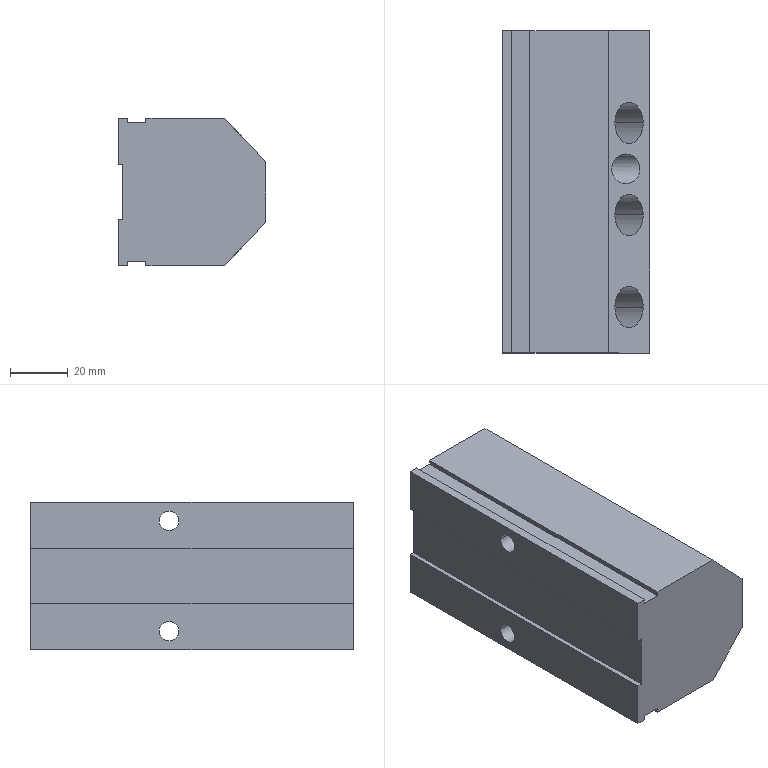Part | STEP file | 4-20.sldasm-Part-24 | 1 solid | 45 faces | box 50.8 x 111.125 x 50.8 mm | volume 204378 mm3 | plane 23 | cylinder 22 | commonest cylinder face diameters 14.287 x6 14.288 x6 6.747 x4 10.319 x4 19.94 x2